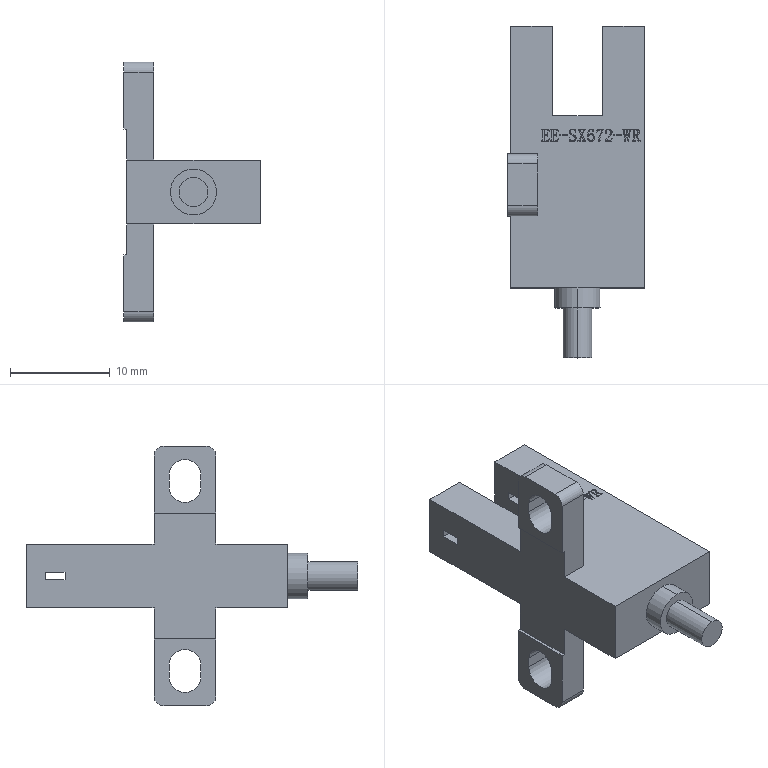Part | STEP file | Sensor OMRON EE-SX672-WR-1 | 1 solid | 290 faces | box 13.7 x 33.2 x 26 mm | volume 2293 mm3 | plane 191 | spline 87 | cylinder 12 | commonest cylinder face diameters 2 x4 3.2 x4 2.9 x2 4.6 x2